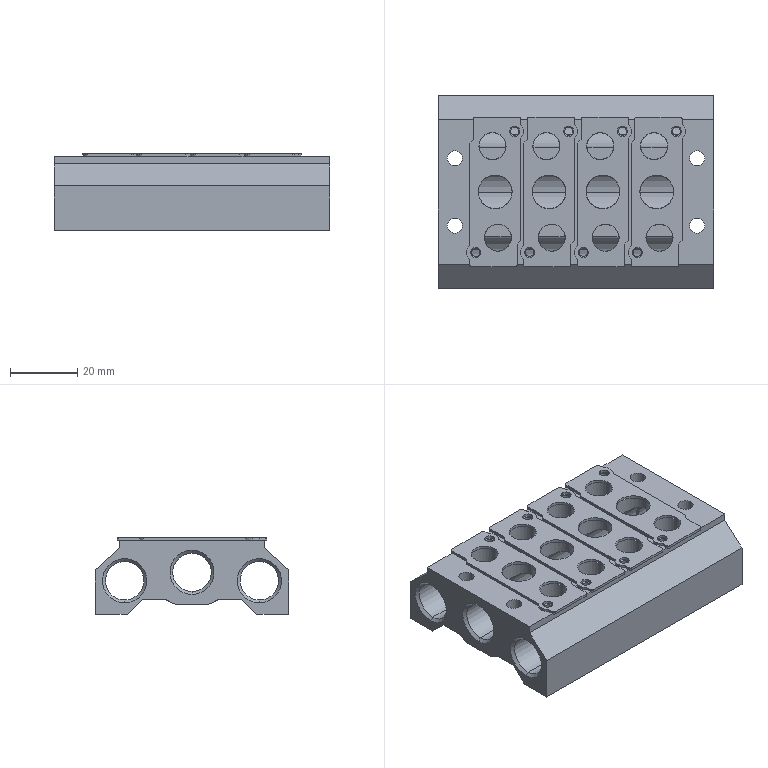Part | SolidWorks | features MBimport 1 | 1 solid | 270 faces | box 82 x 57.5 x 22.8 mm | volume 48619 mm3 | cylinder 134 | plane 108 | cone 28 | commonest cylinder face diameters 1 x16 2.459 x16 3 x16 8 x16 8.05 x16 5.4 x12